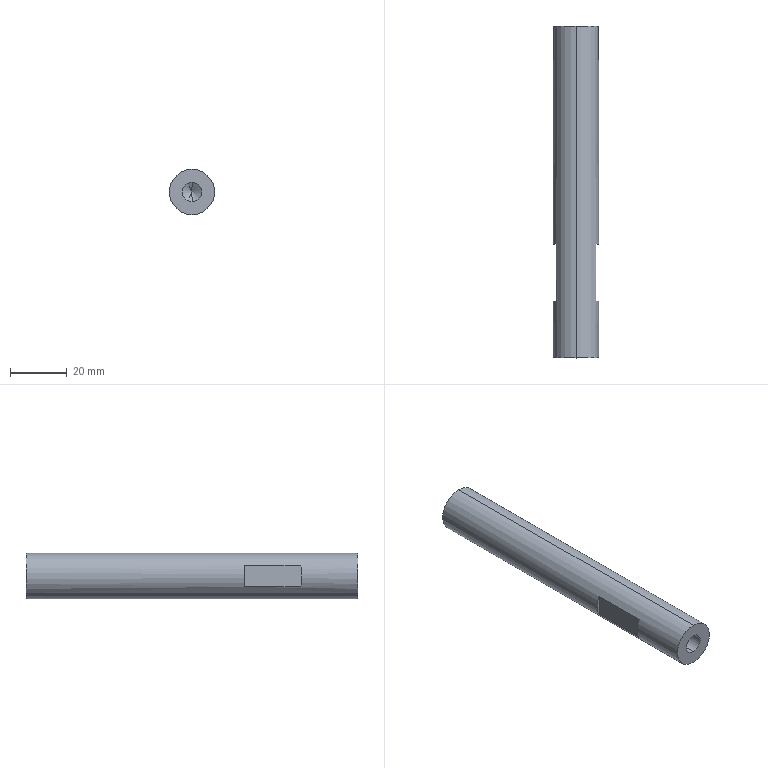Part | STEP file | 1 solid | 18 faces | box 16 x 117 x 16 mm | volume 21831 mm3 | plane 8 | cylinder 6 | cone 4 | commonest cylinder face diameters 6.8 x4 16 x2
STEP:
#1=CARTESIAN_POINT('',(0.,0.,0.));
#2=DIRECTION('',(0.,0.,1.));
#3=DIRECTION('',(1.,0.,0.));
#4=AXIS2_PLACEMENT_3D('',#1,#2,#3);
#5=CARTESIAN_POINT('',(0.,97.25,3.4));
#6=VERTEX_POINT('',#5);
#7=CARTESIAN_POINT('',(0.,117.,3.4));
#8=VERTEX_POINT('',#7);
#9=CARTESIAN_POINT('',(0.,117.,3.4));
#10=DIRECTION('',(0.,1.,0.));
#11=VECTOR('',#10,1.);
#12=LINE('',#9,#11);
#13=CARTESIAN_POINT('',(0.,117.,0.));
#14=DIRECTION('',(0.,1.,0.));
#15=DIRECTION('',(0.,0.,1.));
#16=AXIS2_PLACEMENT_3D('',#13,#14,#15);
#17=CYLINDRICAL_SURFACE('',#16,3.4);
#18=CARTESIAN_POINT('',(6.283,0.));
#19=DIRECTION('',(0.,1.));
#20=VECTOR('',#19,1.);
#21=LINE('',#18,#20);
#22=(GEOMETRIC_REPRESENTATION_CONTEXT(2)PARAMETRIC_REPRESENTATION_CONTEXT()REPRESENTATION_CONTEXT('',''));
#23=DEFINITIONAL_REPRESENTATION('',(#21),#22);
#24=PCURVE('',#17,#23);
#25=CARTESIAN_POINT('',(0.,117.,0.));
#26=DIRECTION('',(0.,1.,0.));
#27=DIRECTION('',(0.,0.,1.));
#28=AXIS2_PLACEMENT_3D('',#25,#26,#27);
#29=CYLINDRICAL_SURFACE('',#28,3.4);
#30=CARTESIAN_POINT('',(0.,0.));
#31=DIRECTION('',(0.,1.));
#32=VECTOR('',#31,1.);
#33=LINE('',#30,#32);
#34=(GEOMETRIC_REPRESENTATION_CONTEXT(2)PARAMETRIC_REPRESENTATION_CONTEXT()REPRESENTATION_CONTEXT('',''));
#35=DEFINITIONAL_REPRESENTATION('',(#33),#34);
#36=PCURVE('',#29,#35);
#37=SURFACE_CURVE('',#12,(#24,#36),.PCURVE_S1.);
#38=EDGE_CURVE('',#6,#8,#37,.T.);
#39=ORIENTED_EDGE('',*,*,#38,.T.);
#40=CARTESIAN_POINT('',(0.,117.,-3.4));
#41=VERTEX_POINT('',#40);
#42=CARTESIAN_POINT('',(0.,117.,0.));
#43=DIRECTION('',(0.,1.,0.));
#44=DIRECTION('',(0.,0.,1.));
#45=AXIS2_PLACEMENT_3D('',#42,#43,#44);
#46=CIRCLE('',#45,3.4);
#47=CARTESIAN_POINT('',(0.,0.));
#48=DIRECTION('',(1.,0.));
#49=VECTOR('',#48,1.);
#50=LINE('',#47,#49);
#51=(GEOMETRIC_REPRESENTATION_CONTEXT(2)PARAMETRIC_REPRESENTATION_CONTEXT()REPRESENTATION_CONTEXT('',''));
#52=DEFINITIONAL_REPRESENTATION('',(#50),#51);
#53=PCURVE('',#17,#52);
#54=CARTESIAN_POINT('',(8.,117.,0.));
#55=DIRECTION('',(0.,1.,0.));
#56=DIRECTION('',(0.,0.,1.));
#57=AXIS2_PLACEMENT_3D('',#54,#55,#56);
#58=PLANE('',#57);
#59=CARTESIAN_POINT('',(0.,-8.));
#60=DIRECTION('',(1.,0.));
#61=AXIS2_PLACEMENT_2D('',#59,#60);
#62=CIRCLE('',#61,3.4);
#63=(GEOMETRIC_REPRESENTATION_CONTEXT(2)PARAMETRIC_REPRESENTATION_CONTEXT()REPRESENTATION_CONTEXT('',''));
#64=DEFINITIONAL_REPRESENTATION('',(#62),#63);
#65=PCURVE('',#58,#64);
#66=SURFACE_CURVE('',#46,(#53,#65),.PCURVE_S1.);
#67=EDGE_CURVE('',#41,#8,#66,.T.);
#68=ORIENTED_EDGE('',*,*,#67,.F.);
#69=CARTESIAN_POINT('',(0.,97.25,-3.4));
#70=VERTEX_POINT('',#69);
#71=CARTESIAN_POINT('',(0.,117.,-3.4));
#72=DIRECTION('',(0.,1.,0.));
#73=VECTOR('',#72,1.);
#74=LINE('',#71,#73);
#75=CARTESIAN_POINT('',(3.142,0.));
#76=DIRECTION('',(0.,1.));
#77=VECTOR('',#76,1.);
#78=LINE('',#75,#77);
#79=(GEOMETRIC_REPRESENTATION_CONTEXT(2)PARAMETRIC_REPRESENTATION_CONTEXT()REPRESENTATION_CONTEXT('',''));
#80=DEFINITIONAL_REPRESENTATION('',(#78),#79);
#81=PCURVE('',#17,#80);
#82=CARTESIAN_POINT('',(3.142,0.));
#83=DIRECTION('',(0.,1.));
#84=VECTOR('',#83,1.);
#85=LINE('',#82,#84);
#86=(GEOMETRIC_REPRESENTATION_CONTEXT(2)PARAMETRIC_REPRESENTATION_CONTEXT()REPRESENTATION_CONTEXT('',''));
#87=DEFINITIONAL_REPRESENTATION('',(#85),#86);
#88=PCURVE('',#29,#87);
#89=SURFACE_CURVE('',#74,(#81,#88),.PCURVE_S1.);
#90=EDGE_CURVE('',#70,#41,#89,.T.);
#91=ORIENTED_EDGE('',*,*,#90,.F.);
#92=CARTESIAN_POINT('',(0.,97.25,0.));
#93=DIRECTION('',(0.,1.,0.));
#94=DIRECTION('',(0.,0.,1.));
#95=AXIS2_PLACEMENT_3D('',#92,#93,#94);
#96=CIRCLE('',#95,3.4);
#97=CARTESIAN_POINT('',(0.,-19.75));
#98=DIRECTION('',(1.,0.));
#99=VECTOR('',#98,1.);
#100=LINE('',#97,#99);
#101=(GEOMETRIC_REPRESENTATION_CONTEXT(2)PARAMETRIC_REPRESENTATION_CONTEXT()REPRESENTATION_CONTEXT('',''));
#102=DEFINITIONAL_REPRESENTATION('',(#100),#101);
#103=PCURVE('',#17,#102);
#104=CARTESIAN_POINT('',(0.,97.25,0.));
#105=DIRECTION('',(0.,1.,0.));
#106=DIRECTION('',(0.,0.,1.));
#107=AXIS2_PLACEMENT_3D('',#104,#105,#106);
#108=CONICAL_SURFACE('',#107,3.4,1.03);
#109=CARTESIAN_POINT('',(0.,0.));
#110=DIRECTION('',(1.,0.));
#111=VECTOR('',#110,1.);
#112=LINE('',#109,#111);
#113=(GEOMETRIC_REPRESENTATION_CONTEXT(2)PARAMETRIC_REPRESENTATION_CONTEXT()REPRESENTATION_CONTEXT('',''));
#114=DEFINITIONAL_REPRESENTATION('',(#112),#113);
#115=PCURVE('',#108,#114);
#116=SURFACE_CURVE('',#96,(#103,#115),.PCURVE_S1.);
#117=EDGE_CURVE('',#70,#6,#116,.T.);
#118=ORIENTED_EDGE('',*,*,#117,.T.);
#119=EDGE_LOOP('',(#39,#68,#91,#118));
#120=FACE_BOUND('',#119,.F.);
#121=ADVANCED_FACE('',(#120),#17,.F.);
#122=ORIENTED_EDGE('',*,*,#117,.F.);
#123=CARTESIAN_POINT('',(0.,95.207,0.));
#124=VERTEX_POINT('',#123);
#125=CARTESIAN_POINT('',(0.,97.25,-3.4));
#126=DIRECTION('',(0.,0.515,-0.8572));
#127=VECTOR('',#126,1.);
#128=LINE('',#125,#127);
#129=CARTESIAN_POINT('',(3.142,-2.043));
#130=CARTESIAN_POINT('',(3.142,-2.012));
#131=CARTESIAN_POINT('',(3.142,-1.95));
#132=CARTESIAN_POINT('',(3.142,-1.857));
#133=CARTESIAN_POINT('',(3.142,-1.764));
#134=CARTESIAN_POINT('',(3.142,-1.671));
#135=CARTESIAN_POINT('',(3.142,-1.579));
#136=CARTESIAN_POINT('',(3.142,-1.486));
#137=CARTESIAN_POINT('',(3.142,-1.393));
#138=CARTESIAN_POINT('',(3.142,-1.3));
#139=CARTESIAN_POINT('',(3.142,-1.207));
#140=CARTESIAN_POINT('',(3.142,-1.114));
#141=CARTESIAN_POINT('',(3.142,-1.021));
#142=CARTESIAN_POINT('',(3.142,-0.9286));
#143=CARTESIAN_POINT('',(3.142,-0.8357));
#144=CARTESIAN_POINT('',(3.142,-0.7429));
#145=CARTESIAN_POINT('',(3.142,-0.65));
#146=CARTESIAN_POINT('',(3.142,-0.5572));
#147=CARTESIAN_POINT('',(3.142,-0.4643));
#148=CARTESIAN_POINT('',(3.142,-0.3714));
#149=CARTESIAN_POINT('',(3.142,-0.2786));
#150=CARTESIAN_POINT('',(3.142,-0.1857));
#151=CARTESIAN_POINT('',(3.142,-0.09286));
#152=CARTESIAN_POINT('',(3.142,-0.03095));
#153=CARTESIAN_POINT('',(3.142,0.));
#154=B_SPLINE_CURVE_WITH_KNOTS('',3,(#129,#130,#131,#132,#133,#134,#135,#136,#137,#138,#139,#140,#141,#142,#143,#144,#145,#146,#147,#148,#149,#150,#151,#152,#153),.UNSPECIFIED.,.F.,.F.,(4,1,1,1,1,1,1,1,1,1,1,1,1,1,1,1,1,1,1,1,1,1,4),(-3.967,-3.786,-3.606,-3.426,-3.245,-3.065,-2.885,-2.704,-2.524,-2.344,-2.164,-1.983,-1.803,-1.623,-1.442,-1.262,-1.082,-0.9015,-0.7212,-0.5409,-0.3606,-0.1803,0.),.UNSPECIFIED.);
#155=(GEOMETRIC_REPRESENTATION_CONTEXT(2)PARAMETRIC_REPRESENTATION_CONTEXT()REPRESENTATION_CONTEXT('',''));
#156=DEFINITIONAL_REPRESENTATION('',(#154),#155);
#157=PCURVE('',#108,#156);
#158=CARTESIAN_POINT('',(0.,97.25,0.));
#159=DIRECTION('',(0.,1.,0.));
#160=DIRECTION('',(0.,0.,1.));
#161=AXIS2_PLACEMENT_3D('',#158,#159,#160);
#162=CONICAL_SURFACE('',#161,3.4,1.03);
#163=CARTESIAN_POINT('',(3.142,-2.043));
#164=CARTESIAN_POINT('',(3.142,-2.012));
#165=CARTESIAN_POINT('',(3.142,-1.95));
#166=CARTESIAN_POINT('',(3.142,-1.857));
#167=CARTESIAN_POINT('',(3.142,-1.764));
#168=CARTESIAN_POINT('',(3.142,-1.671));
#169=CARTESIAN_POINT('',(3.142,-1.579));
#170=CARTESIAN_POINT('',(3.142,-1.486));
#171=CARTESIAN_POINT('',(3.142,-1.393));
#172=CARTESIAN_POINT('',(3.142,-1.3));
#173=CARTESIAN_POINT('',(3.142,-1.207));
#174=CARTESIAN_POINT('',(3.142,-1.114));
#175=CARTESIAN_POINT('',(3.142,-1.021));
#176=CARTESIAN_POINT('',(3.142,-0.9286));
#177=CARTESIAN_POINT('',(3.142,-0.8357));
#178=CARTESIAN_POINT('',(3.142,-0.7429));
#179=CARTESIAN_POINT('',(3.142,-0.65));
#180=CARTESIAN_POINT('',(3.142,-0.5572));
#181=CARTESIAN_POINT('',(3.142,-0.4643));
#182=CARTESIAN_POINT('',(3.142,-0.3714));
#183=CARTESIAN_POINT('',(3.142,-0.2786));
#184=CARTESIAN_POINT('',(3.142,-0.1857));
#185=CARTESIAN_POINT('',(3.142,-0.09286));
#186=CARTESIAN_POINT('',(3.142,-0.03095));
#187=CARTESIAN_POINT('',(3.142,0.));
#188=B_SPLINE_CURVE_WITH_KNOTS('',3,(#163,#164,#165,#166,#167,#168,#169,#170,#171,#172,#173,#174,#175,#176,#177,#178,#179,#180,#181,#182,#183,#184,#185,#186,#187),.UNSPECIFIED.,.F.,.F.,(4,1,1,1,1,1,1,1,1,1,1,1,1,1,1,1,1,1,1,1,1,1,4),(-3.967,-3.786,-3.606,-3.426,-3.245,-3.065,-2.885,-2.704,-2.524,-2.344,-2.164,-1.983,-1.803,-1.623,-1.442,-1.262,-1.082,-0.9015,-0.7212,-0.5409,-0.3606,-0.1803,0.),.UNSPECIFIED.);
#189=(GEOMETRIC_REPRESENTATION_CONTEXT(2)PARAMETRIC_REPRESENTATION_CONTEXT()REPRESENTATION_CONTEXT('',''));
#190=DEFINITIONAL_REPRESENTATION('',(#188),#189);
#191=PCURVE('',#162,#190);
#192=SURFACE_CURVE('',#128,(#157,#191),.PCURVE_S1.);
#193=EDGE_CURVE('',#124,#70,#192,.T.);
#194=ORIENTED_EDGE('',*,*,#193,.F.);
#195=CARTESIAN_POINT('',(0.,97.25,3.4));
#196=DIRECTION('',(0.,0.515,0.8572));
#197=VECTOR('',#196,1.);
#198=LINE('',#195,#197);
#199=CARTESIAN_POINT('',(6.283,-2.043));
#200=CARTESIAN_POINT('',(6.283,-2.012));
#201=CARTESIAN_POINT('',(6.283,-1.95));
#202=CARTESIAN_POINT('',(6.283,-1.857));
#203=CARTESIAN_POINT('',(6.283,-1.764));
#204=CARTESIAN_POINT('',(6.283,-1.671));
#205=CARTESIAN_POINT('',(6.283,-1.579));
#206=CARTESIAN_POINT('',(6.283,-1.486));
#207=CARTESIAN_POINT('',(6.283,-1.393));
#208=CARTESIAN_POINT('',(6.283,-1.3));
#209=CARTESIAN_POINT('',(6.283,-1.207));
#210=CARTESIAN_POINT('',(6.283,-1.114));
#211=CARTESIAN_POINT('',(6.283,-1.021));
#212=CARTESIAN_POINT('',(6.283,-0.9286));
#213=CARTESIAN_POINT('',(6.283,-0.8357));
#214=CARTESIAN_POINT('',(6.283,-0.7429));
#215=CARTESIAN_POINT('',(6.283,-0.65));
#216=CARTESIAN_POINT('',(6.283,-0.5572));
#217=CARTESIAN_POINT('',(6.283,-0.4643));
#218=CARTESIAN_POINT('',(6.283,-0.3714));
#219=CARTESIAN_POINT('',(6.283,-0.2786));
#220=CARTESIAN_POINT('',(6.283,-0.1857));
#221=CARTESIAN_POINT('',(6.283,-0.09286));
#222=CARTESIAN_POINT('',(6.283,-0.03095));
#223=CARTESIAN_POINT('',(6.283,0.));
#224=B_SPLINE_CURVE_WITH_KNOTS('',3,(#199,#200,#201,#202,#203,#204,#205,#206,#207,#208,#209,#210,#211,#212,#213,#214,#215,#216,#217,#218,#219,#220,#221,#222,#223),.UNSPECIFIED.,.F.,.F.,(4,1,1,1,1,1,1,1,1,1,1,1,1,1,1,1,1,1,1,1,1,1,4),(-3.967,-3.786,-3.606,-3.426,-3.245,-3.065,-2.885,-2.704,-2.524,-2.344,-2.164,-1.983,-1.803,-1.623,-1.442,-1.262,-1.082,-0.9015,-0.7212,-0.5409,-0.3606,-0.1803,0.),.UNSPECIFIED.);
#225=(GEOMETRIC_REPRESENTATION_CONTEXT(2)PARAMETRIC_REPRESENTATION_CONTEXT()REPRESENTATION_CONTEXT('',''));
#226=DEFINITIONAL_REPRESENTATION('',(#224),#225);
#227=PCURVE('',#108,#226);
#228=CARTESIAN_POINT('',(0.,-2.043));
#229=CARTESIAN_POINT('',(0.,-2.012));
#230=CARTESIAN_POINT('',(0.,-1.95));
#231=CARTESIAN_POINT('',(0.,-1.857));
#232=CARTESIAN_POINT('',(0.,-1.764));
#233=CARTESIAN_POINT('',(0.,-1.671));
#234=CARTESIAN_POINT('',(0.,-1.579));
#235=CARTESIAN_POINT('',(0.,-1.486));
#236=CARTESIAN_POINT('',(0.,-1.393));
#237=CARTESIAN_POINT('',(0.,-1.3));
#238=CARTESIAN_POINT('',(0.,-1.207));
#239=CARTESIAN_POINT('',(0.,-1.114));
#240=CARTESIAN_POINT('',(0.,-1.021));
#241=CARTESIAN_POINT('',(0.,-0.9286));
#242=CARTESIAN_POINT('',(0.,-0.8357));
#243=CARTESIAN_POINT('',(0.,-0.7429));
#244=CARTESIAN_POINT('',(0.,-0.65));
#245=CARTESIAN_POINT('',(0.,-0.5572));
#246=CARTESIAN_POINT('',(0.,-0.4643));
#247=CARTESIAN_POINT('',(0.,-0.3714));
#248=CARTESIAN_POINT('',(0.,-0.2786));
#249=CARTESIAN_POINT('',(0.,-0.1857));
#250=CARTESIAN_POINT('',(0.,-0.09286));
#251=CARTESIAN_POINT('',(0.,-0.03095));
#252=CARTESIAN_POINT('',(0.,0.));
#253=B_SPLINE_CURVE_WITH_KNOTS('',3,(#228,#229,#230,#231,#232,#233,#234,#235,#236,#237,#238,#239,#240,#241,#242,#243,#244,#245,#246,#247,#248,#249,#250,#251,#252),.UNSPECIFIED.,.F.,.F.,(4,1,1,1,1,1,1,1,1,1,1,1,1,1,1,1,1,1,1,1,1,1,4),(-3.967,-3.786,-3.606,-3.426,-3.245,-3.065,-2.885,-2.704,-2.524,-2.344,-2.164,-1.983,-1.803,-1.623,-1.442,-1.262,-1.082,-0.9015,-0.7212,-0.5409,-0.3606,-0.1803,0.),.UNSPECIFIED.);
#254=(GEOMETRIC_REPRESENTATION_CONTEXT(2)PARAMETRIC_REPRESENTATION_CONTEXT()REPRESENTATION_CONTEXT('',''));
#255=DEFINITIONAL_REPRESENTATION('',(#253),#254);
#256=PCURVE('',#162,#255);
#257=SURFACE_CURVE('',#198,(#227,#256),.PCURVE_S1.);
#258=EDGE_CURVE('',#124,#6,#257,.T.);
#259=ORIENTED_EDGE('',*,*,#258,.T.);
#260=EDGE_LOOP('',(#122,#194,#259));
#261=FACE_BOUND('',#260,.F.);
#262=ADVANCED_FACE('',(#261),#108,.F.);
#263=CARTESIAN_POINT('',(0.,19.75,-3.4));
#264=VERTEX_POINT('',#263);
#265=CARTESIAN_POINT('',(0.,0.,-3.4));
#266=VERTEX_POINT('',#265);
#267=CARTESIAN_POINT('',(0.,0.,-3.4));
#268=DIRECTION('',(0.,-1.,0.));
#269=VECTOR('',#268,1.);
#270=LINE('',#267,#269);
#271=CARTESIAN_POINT('',(0.,0.,0.));
#272=DIRECTION('',(0.,-1.,0.));
#273=DIRECTION('',(0.,0.,-1.));
#274=AXIS2_PLACEMENT_3D('',#271,#272,#273);
#275=CYLINDRICAL_SURFACE('',#274,3.4);
#276=CARTESIAN_POINT('',(6.283,0.));
#277=DIRECTION('',(0.,1.));
#278=VECTOR('',#277,1.);
#279=LINE('',#276,#278);
#280=(GEOMETRIC_REPRESENTATION_CONTEXT(2)PARAMETRIC_REPRESENTATION_CONTEXT()REPRESENTATION_CONTEXT('',''));
#281=DEFINITIONAL_REPRESENTATION('',(#279),#280);
#282=PCURVE('',#275,#281);
#283=CARTESIAN_POINT('',(0.,0.,0.));
#284=DIRECTION('',(0.,-1.,0.));
#285=DIRECTION('',(0.,0.,-1.));
#286=AXIS2_PLACEMENT_3D('',#283,#284,#285);
#287=CYLINDRICAL_SURFACE('',#286,3.4);
#288=CARTESIAN_POINT('',(0.,0.));
#289=DIRECTION('',(0.,1.));
#290=VECTOR('',#289,1.);
#291=LINE('',#288,#290);
#292=(GEOMETRIC_REPRESENTATION_CONTEXT(2)PARAMETRIC_REPRESENTATION_CONTEXT()REPRESENTATION_CONTEXT('',''));
#293=DEFINITIONAL_REPRESENTATION('',(#291),#292);
#294=PCURVE('',#287,#293);
#295=SURFACE_CURVE('',#270,(#282,#294),.PCURVE_S1.);
#296=EDGE_CURVE('',#264,#266,#295,.T.);
#297=ORIENTED_EDGE('',*,*,#296,.T.);
#298=CARTESIAN_POINT('',(0.,0.,3.4));
#299=VERTEX_POINT('',#298);
#300=CARTESIAN_POINT('',(0.,0.,0.));
#301=DIRECTION('',(0.,-1.,0.));
#302=DIRECTION('',(0.,0.,-1.));
#303=AXIS2_PLACEMENT_3D('',#300,#301,#302);
#304=CIRCLE('',#303,3.4);
#305=CARTESIAN_POINT('',(0.,0.));
#306=DIRECTION('',(1.,0.));
#307=VECTOR('',#306,1.);
#308=LINE('',#305,#307);
#309=(GEOMETRIC_REPRESENTATION_CONTEXT(2)PARAMETRIC_REPRESENTATION_CONTEXT()REPRESENTATION_CONTEXT('',''));
#310=DEFINITIONAL_REPRESENTATION('',(#308),#309);
#311=PCURVE('',#275,#310);
#312=CARTESIAN_POINT('',(0.,0.,0.));
#313=DIRECTION('',(0.,-1.,0.));
#314=DIRECTION('',(0.,0.,-1.));
#315=AXIS2_PLACEMENT_3D('',#312,#313,#314);
#316=PLANE('',#315);
#317=CARTESIAN_POINT('',(0.,0.));
#318=DIRECTION('',(1.,0.));
#319=AXIS2_PLACEMENT_2D('',#317,#318);
#320=CIRCLE('',#319,3.4);
#321=(GEOMETRIC_REPRESENTATION_CONTEXT(2)PARAMETRIC_REPRESENTATION_CONTEXT()REPRESENTATION_CONTEXT('',''));
#322=DEFINITIONAL_REPRESENTATION('',(#320),#321);
#323=PCURVE('',#316,#322);
#324=SURFACE_CURVE('',#304,(#311,#323),.PCURVE_S1.);
#325=EDGE_CURVE('',#299,#266,#324,.T.);
#326=ORIENTED_EDGE('',*,*,#325,.F.);
#327=CARTESIAN_POINT('',(0.,19.75,3.4));
#328=VERTEX_POINT('',#327);
#329=CARTESIAN_POINT('',(0.,0.,3.4));
#330=DIRECTION('',(0.,-1.,0.));
#331=VECTOR('',#330,1.);
#332=LINE('',#329,#331);
#333=CARTESIAN_POINT('',(3.142,0.));
#334=DIRECTION('',(0.,1.));
#335=VECTOR('',#334,1.);
#336=LINE('',#333,#335);
#337=(GEOMETRIC_REPRESENTATION_CONTEXT(2)PARAMETRIC_REPRESENTATION_CONTEXT()REPRESENTATION_CONTEXT('',''));
#338=DEFINITIONAL_REPRESENTATION('',(#336),#337);
#339=PCURVE('',#275,#338);
#340=CARTESIAN_POINT('',(3.142,0.));
#341=DIRECTION('',(0.,1.));
#342=VECTOR('',#341,1.);
#343=LINE('',#340,#342);
#344=(GEOMETRIC_REPRESENTATION_CONTEXT(2)PARAMETRIC_REPRESENTATION_CONTEXT()REPRESENTATION_CONTEXT('',''));
#345=DEFINITIONAL_REPRESENTATION('',(#343),#344);
#346=PCURVE('',#287,#345);
#347=SURFACE_CURVE('',#332,(#339,#346),.PCURVE_S1.);
#348=EDGE_CURVE('',#328,#299,#347,.T.);
#349=ORIENTED_EDGE('',*,*,#348,.F.);
#350=CARTESIAN_POINT('',(0.,19.75,0.));
#351=DIRECTION('',(0.,-1.,0.));
#352=DIRECTION('',(0.,0.,-1.));
#353=AXIS2_PLACEMENT_3D('',#350,#351,#352);
#354=CIRCLE('',#353,3.4);
#355=CARTESIAN_POINT('',(0.,-19.75));
#356=DIRECTION('',(1.,0.));
#357=VECTOR('',#356,1.);
#358=LINE('',#355,#357);
#359=(GEOMETRIC_REPRESENTATION_CONTEXT(2)PARAMETRIC_REPRESENTATION_CONTEXT()REPRESENTATION_CONTEXT('',''));
#360=DEFINITIONAL_REPRESENTATION('',(#358),#359);
#361=PCURVE('',#275,#360);
#362=CARTESIAN_POINT('',(0.,19.75,0.));
#363=DIRECTION('',(0.,-1.,0.));
#364=DIRECTION('',(0.,0.,-1.));
#365=AXIS2_PLACEMENT_3D('',#362,#363,#364);
#366=CONICAL_SURFACE('',#365,3.4,1.03);
#367=CARTESIAN_POINT('',(0.,0.));
#368=DIRECTION('',(1.,0.));
#369=VECTOR('',#368,1.);
#370=LINE('',#367,#369);
#371=(GEOMETRIC_REPRESENTATION_CONTEXT(2)PARAMETRIC_REPRESENTATION_CONTEXT()REPRESENTATION_CONTEXT('',''));
#372=DEFINITIONAL_REPRESENTATION('',(#370),#371);
#373=PCURVE('',#366,#372);
#374=SURFACE_CURVE('',#354,(#361,#373),.PCURVE_S1.);
#375=EDGE_CURVE('',#328,#264,#374,.T.);
#376=ORIENTED_EDGE('',*,*,#375,.T.);
#377=EDGE_LOOP('',(#297,#326,#349,#376));
#378=FACE_BOUND('',#377,.F.);
#379=ADVANCED_FACE('',(#378),#275,.F.);
#380=ORIENTED_EDGE('',*,*,#375,.F.);
#381=CARTESIAN_POINT('',(0.,21.793,0.));
#382=VERTEX_POINT('',#381);
#383=CARTESIAN_POINT('',(0.,19.75,3.4));
#384=DIRECTION('',(0.,-0.515,0.8572));
#385=VECTOR('',#384,1.);
#386=LINE('',#383,#385);
#387=CARTESIAN_POINT('',(3.142,-2.043));
#388=CARTESIAN_POINT('',(3.142,-2.012));
#389=CARTESIAN_POINT('',(3.142,-1.95));
#390=CARTESIAN_POINT('',(3.142,-1.857));
#391=CARTESIAN_POINT('',(3.142,-1.764));
#392=CARTESIAN_POINT('',(3.142,-1.671));
#393=CARTESIAN_POINT('',(3.142,-1.579));
#394=CARTESIAN_POINT('',(3.142,-1.486));
#395=CARTESIAN_POINT('',(3.142,-1.393));
#396=CARTESIAN_POINT('',(3.142,-1.3));
#397=CARTESIAN_POINT('',(3.142,-1.207));
#398=CARTESIAN_POINT('',(3.142,-1.114));
#399=CARTESIAN_POINT('',(3.142,-1.021));
#400=CARTESIAN_POINT('',(3.142,-0.9286));
#401=CARTESIAN_POINT('',(3.142,-0.8357));
#402=CARTESIAN_POINT('',(3.142,-0.7429));
#403=CARTESIAN_POINT('',(3.142,-0.65));
#404=CARTESIAN_POINT('',(3.142,-0.5572));
#405=CARTESIAN_POINT('',(3.142,-0.4643));
#406=CARTESIAN_POINT('',(3.142,-0.3714));
#407=CARTESIAN_POINT('',(3.142,-0.2786));
#408=CARTESIAN_POINT('',(3.142,-0.1857));
#409=CARTESIAN_POINT('',(3.142,-0.09286));
#410=CARTESIAN_POINT('',(3.142,-0.03095));
#411=CARTESIAN_POINT('',(3.142,0.));
#412=B_SPLINE_CURVE_WITH_KNOTS('',3,(#387,#388,#389,#390,#391,#392,#393,#394,#395,#396,#397,#398,#399,#400,#401,#402,#403,#404,#405,#406,#407,#408,#409,#410,#411),.UNSPECIFIED.,.F.,.F.,(4,1,1,1,1,1,1,1,1,1,1,1,1,1,1,1,1,1,1,1,1,1,4),(-3.967,-3.786,-3.606,-3.426,-3.245,-3.065,-2.885,-2.704,-2.524,-2.344,-2.164,-1.983,-1.803,-1.623,-1.442,-1.262,-1.082,-0.9015,-0.7212,-0.5409,-0.3606,-0.1803,0.),.QUASI_UNIFORM_KNOTS.);
#413=(GEOMETRIC_REPRESENTATION_CONTEXT(2)PARAMETRIC_REPRESENTATION_CONTEXT()REPRESENTATION_CONTEXT('',''));
#414=DEFINITIONAL_REPRESENTATION('',(#412),#413);
#415=PCURVE('',#366,#414);
#416=CARTESIAN_POINT('',(0.,19.75,0.));
#417=DIRECTION('',(0.,-1.,0.));
#418=DIRECTION('',(0.,0.,-1.));
#419=AXIS2_PLACEMENT_3D('',#416,#417,#418);
#420=CONICAL_SURFACE('',#419,3.4,1.03);
#421=CARTESIAN_POINT('',(3.142,-2.043));
#422=CARTESIAN_POINT('',(3.142,-2.012));
#423=CARTESIAN_POINT('',(3.142,-1.95));
#424=CARTESIAN_POINT('',(3.142,-1.857));
#425=CARTESIAN_POINT('',(3.142,-1.764));
#426=CARTESIAN_POINT('',(3.142,-1.671));
#427=CARTESIAN_POINT('',(3.142,-1.579));
#428=CARTESIAN_POINT('',(3.142,-1.486));
#429=CARTESIAN_POINT('',(3.142,-1.393));
#430=CARTESIAN_POINT('',(3.142,-1.3));
#431=CARTESIAN_POINT('',(3.142,-1.207));
#432=CARTESIAN_POINT('',(3.142,-1.114));
#433=CARTESIAN_POINT('',(3.142,-1.021));
#434=CARTESIAN_POINT('',(3.142,-0.9286));
#435=CARTESIAN_POINT('',(3.142,-0.8357));
#436=CARTESIAN_POINT('',(3.142,-0.7429));
#437=CARTESIAN_POINT('',(3.142,-0.65));
#438=CARTESIAN_POINT('',(3.142,-0.5572));
#439=CARTESIAN_POINT('',(3.142,-0.4643));
#440=CARTESIAN_POINT('',(3.142,-0.3714));
#441=CARTESIAN_POINT('',(3.142,-0.2786));
#442=CARTESIAN_POINT('',(3.142,-0.1857));
#443=CARTESIAN_POINT('',(3.142,-0.09286));
#444=CARTESIAN_POINT('',(3.142,-0.03095));
#445=CARTESIAN_POINT('',(3.142,0.));
#446=B_SPLINE_CURVE_WITH_KNOTS('',3,(#421,#422,#423,#424,#425,#426,#427,#428,#429,#430,#431,#432,#433,#434,#435,#436,#437,#438,#439,#440,#441,#442,#443,#444,#445),.UNSPECIFIED.,.F.,.F.,(4,1,1,1,1,1,1,1,1,1,1,1,1,1,1,1,1,1,1,1,1,1,4),(-3.967,-3.786,-3.606,-3.426,-3.245,-3.065,-2.885,-2.704,-2.524,-2.344,-2.164,-1.983,-1.803,-1.623,-1.442,-1.262,-1.082,-0.9015,-0.7212,-0.5409,-0.3606,-0.1803,0.),.QUASI_UNIFORM_KNOTS.);
#447=(GEOMETRIC_REPRESENTATION_CONTEXT(2)PARAMETRIC_REPRESENTATION_CONTEXT()REPRESENTATION_CONTEXT('',''));
#448=DEFINITIONAL_REPRESENTATION('',(#446),#447);
#449=PCURVE('',#420,#448);
#450=SURFACE_CURVE('',#386,(#415,#449),.PCURVE_S1.);
#451=EDGE_CURVE('',#382,#328,#450,.T.);
#452=ORIENTED_EDGE('',*,*,#451,.F.);
#453=CARTESIAN_POINT('',(0.,19.75,-3.4));
#454=DIRECTION('',(0.,-0.515,-0.8572));
#455=VECTOR('',#454,1.);
#456=LINE('',#453,#455);
#457=CARTESIAN_POINT('',(6.283,-2.043));
#458=CARTESIAN_POINT('',(6.283,-2.012));
#459=CARTESIAN_POINT('',(6.283,-1.95));
#460=CARTESIAN_POINT('',(6.283,-1.857));
#461=CARTESIAN_POINT('',(6.283,-1.764));
#462=CARTESIAN_POINT('',(6.283,-1.671));
#463=CARTESIAN_POINT('',(6.283,-1.579));
#464=CARTESIAN_POINT('',(6.283,-1.486));
#465=CARTESIAN_POINT('',(6.283,-1.393));
#466=CARTESIAN_POINT('',(6.283,-1.3));
#467=CARTESIAN_POINT('',(6.283,-1.207));
#468=CARTESIAN_POINT('',(6.283,-1.114));
#469=CARTESIAN_POINT('',(6.283,-1.021));
#470=CARTESIAN_POINT('',(6.283,-0.9286));
#471=CARTESIAN_POINT('',(6.283,-0.8357));
#472=CARTESIAN_POINT('',(6.283,-0.7429));
#473=CARTESIAN_POINT('',(6.283,-0.65));
#474=CARTESIAN_POINT('',(6.283,-0.5572));
#475=CARTESIAN_POINT('',(6.283,-0.4643));
#476=CARTESIAN_POINT('',(6.283,-0.3714));
#477=CARTESIAN_POINT('',(6.283,-0.2786));
#478=CARTESIAN_POINT('',(6.283,-0.1857));
#479=CARTESIAN_POINT('',(6.283,-0.09286));
#480=CARTESIAN_POINT('',(6.283,-0.03095));
#481=CARTESIAN_POINT('',(6.283,0.));
#482=B_SPLINE_CURVE_WITH_KNOTS('',3,(#457,#458,#459,#460,#461,#462,#463,#464,#465,#466,#467,#468,#469,#470,#471,#472,#473,#474,#475,#476,#477,#478,#479,#480,#481),.UNSPECIFIED.,.F.,.F.,(4,1,1,1,1,1,1,1,1,1,1,1,1,1,1,1,1,1,1,1,1,1,4),(-3.967,-3.786,-3.606,-3.426,-3.245,-3.065,-2.885,-2.704,-2.524,-2.344,-2.164,-1.983,-1.803,-1.623,-1.442,-1.262,-1.082,-0.9015,-0.7212,-0.5409,-0.3606,-0.1803,0.),.QUASI_UNIFORM_KNOTS.);
#483=(GEOMETRIC_REPRESENTATION_CONTEXT(2)PARAMETRIC_REPRESENTATION_CONTEXT()REPRESENTATION_CONTEXT('',''));
#484=DEFINITIONAL_REPRESENTATION('',(#482),#483);
#485=PCURVE('',#366,#484);
#486=CARTESIAN_POINT('',(0.,-2.043));
#487=CARTESIAN_POINT('',(0.,-2.012));
#488=CARTESIAN_POINT('',(0.,-1.95));
#489=CARTESIAN_POINT('',(0.,-1.857));
#490=CARTESIAN_POINT('',(0.,-1.764));
#491=CARTESIAN_POINT('',(0.,-1.671));
#492=CARTESIAN_POINT('',(0.,-1.579));
#493=CARTESIAN_POINT('',(0.,-1.486));
#494=CARTESIAN_POINT('',(0.,-1.393));
#495=CARTESIAN_POINT('',(0.,-1.3));
#496=CARTESIAN_POINT('',(0.,-1.207));
#497=CARTESIAN_POINT('',(0.,-1.114));
#498=CARTESIAN_POINT('',(0.,-1.021));
#499=CARTESIAN_POINT('',(0.,-0.9286));
#500=CARTESIAN_POINT('',(0.,-0.8357));
#501=CARTESIAN_POINT('',(0.,-0.7429));
#502=CARTESIAN_POINT('',(0.,-0.65));
#503=CARTESIAN_POINT('',(0.,-0.5572));
#504=CARTESIAN_POINT('',(0.,-0.4643));
#505=CARTESIAN_POINT('',(0.,-0.3714));
#506=CARTESIAN_POINT('',(0.,-0.2786));
#507=CARTESIAN_POINT('',(0.,-0.1857));
#508=CARTESIAN_POINT('',(0.,-0.09286));
#509=CARTESIAN_POINT('',(0.,-0.03095));
#510=CARTESIAN_POINT('',(0.,0.));
#511=B_SPLINE_CURVE_WITH_KNOTS('',3,(#486,#487,#488,#489,#490,#491,#492,#493,#494,#495,#496,#497,#498,#499,#500,#501,#502,#503,#504,#505,#506,#507,#508,#509,#510),.UNSPECIFIED.,.F.,.F.,(4,1,1,1,1,1,1,1,1,1,1,1,1,1,1,1,1,1,1,1,1,1,4),(-3.967,-3.786,-3.606,-3.426,-3.245,-3.065,-2.885,-2.704,-2.524,-2.344,-2.164,-1.983,-1.803,-1.623,-1.442,-1.262,-1.082,-0.9015,-0.7212,-0.5409,-0.3606,-0.1803,0.),.QUASI_UNIFORM_KNOTS.);
#512=(GEOMETRIC_REPRESENTATION_CONTEXT(2)PARAMETRIC_REPRESENTATION_CONTEXT()REPRESENTATION_CONTEXT('',''));
#513=DEFINITIONAL_REPRESENTATION('',(#511),#512);
#514=PCURVE('',#420,#513);
#515=SURFACE_CURVE('',#456,(#485,#514),.PCURVE_S1.);
#516=EDGE_CURVE('',#382,#264,#515,.T.);
#517=ORIENTED_EDGE('',*,*,#516,.T.);
#518=EDGE_LOOP('',(#380,#452,#517));
#519=FACE_BOUND('',#518,.F.);
#520=ADVANCED_FACE('',(#519),#366,.F.);
#521=CARTESIAN_POINT('',(7.,20.,3.873));
#522=VERTEX_POINT('',#521);
#523=CARTESIAN_POINT('',(7.,20.,-3.873));
#524=VERTEX_POINT('',#523);
#525=CARTESIAN_POINT('',(0.,20.,0.));
#526=DIRECTION('',(0.,1.,0.));
#527=DIRECTION('',(1.,0.,0.));
#528=AXIS2_PLACEMENT_3D('',#525,#526,#527);
#529=CIRCLE('',#528,8.);
#530=CARTESIAN_POINT('',(0.,0.,0.));
#531=DIRECTION('',(0.,-1.,0.));
#532=DIRECTION('',(0.,0.,-1.));
#533=AXIS2_PLACEMENT_3D('',#530,#531,#532);
#534=CYLINDRICAL_SURFACE('',#533,8.);
#535=CARTESIAN_POINT('',(7.854,-20.));
#536=DIRECTION('',(-1.,0.));
#537=VECTOR('',#536,1.);
#538=LINE('',#535,#537);
#539=(GEOMETRIC_REPRESENTATION_CONTEXT(2)PARAMETRIC_REPRESENTATION_CONTEXT()REPRESENTATION_CONTEXT('',''));
#540=DEFINITIONAL_REPRESENTATION('',(#538),#539);
#541=PCURVE('',#534,#540);
#542=CARTESIAN_POINT('',(13.,20.,-10.));
#543=DIRECTION('',(0.,-1.,0.));
#544=DIRECTION('',(1.,0.,0.));
#545=AXIS2_PLACEMENT_3D('',#542,#543,#544);
#546=PLANE('',#545);
#547=CARTESIAN_POINT('',(-5.,10.));
#548=CARTESIAN_POINT('',(-5.,-3.856));
#549=CARTESIAN_POINT('',(-17.,3.072));
#550=CARTESIAN_POINT('',(-29.,10.));
#551=CARTESIAN_POINT('',(-17.,16.928));
#552=CARTESIAN_POINT('',(-5.,23.856));
#553=CARTESIAN_POINT('',(-5.,10.));
#554=(BOUNDED_CURVE()B_SPLINE_CURVE(2,(#547,#548,#549,#550,#551,#552,#553),.UNSPECIFIED.,.T.,.F.)B_SPLINE_CURVE_WITH_KNOTS((1,2,2,2,2,1),(-2.094,0.,2.094,4.189,6.283,8.378),.UNSPECIFIED.)CURVE()GEOMETRIC_REPRESENTATION_ITEM()RATIONAL_B_SPLINE_CURVE((1.,0.5,1.,0.5,1.,0.5,1.))REPRESENTATION_ITEM(''));
#555=(GEOMETRIC_REPRESENTATION_CONTEXT(2)PARAMETRIC_REPRESENTATION_CONTEXT()REPRESENTATION_CONTEXT('',''));
#556=DEFINITIONAL_REPRESENTATION('',(#554),#555);
#557=PCURVE('',#546,#556);
#558=SURFACE_CURVE('',#529,(#541,#557),.PCURVE_S1.);
#559=EDGE_CURVE('',#522,#524,#558,.T.);
#560=ORIENTED_EDGE('',*,*,#559,.F.);
#561=CARTESIAN_POINT('',(7.,40.,3.873));
#562=VERTEX_POINT('',#561);
#563=CARTESIAN_POINT('',(7.,0.,3.873));
#564=DIRECTION('',(0.,-1.,0.));
#565=VECTOR('',#564,1.);
#566=LINE('',#563,#565);
#567=CARTESIAN_POINT('',(2.076,0.));
#568=DIRECTION('',(0.,1.));
#569=VECTOR('',#568,1.);
#570=LINE('',#567,#569);
#571=(GEOMETRIC_REPRESENTATION_CONTEXT(2)PARAMETRIC_REPRESENTATION_CONTEXT()REPRESENTATION_CONTEXT('',''));
#572=DEFINITIONAL_REPRESENTATION('',(#570),#571);
#573=PCURVE('',#534,#572);
#574=CARTESIAN_POINT('',(7.,20.,-10.));
#575=DIRECTION('',(-1.,0.,0.));
#576=DIRECTION('',(0.,0.,1.));
#577=AXIS2_PLACEMENT_3D('',#574,#575,#576);
#578=PLANE('',#577);
#579=CARTESIAN_POINT('',(13.873,-20.));
#580=DIRECTION('',(0.,-1.));
#581=VECTOR('',#580,1.);
#582=LINE('',#579,#581);
#583=(GEOMETRIC_REPRESENTATION_CONTEXT(2)PARAMETRIC_REPRESENTATION_CONTEXT()REPRESENTATION_CONTEXT('',''));
#584=DEFINITIONAL_REPRESENTATION('',(#582),#583);
#585=PCURVE('',#578,#584);
#586=SURFACE_CURVE('',#566,(#573,#585),.PCURVE_S1.);
#587=EDGE_CURVE('',#562,#522,#586,.T.);
#588=ORIENTED_EDGE('',*,*,#587,.F.);
#589=CARTESIAN_POINT('',(7.,40.,-3.873));
#590=VERTEX_POINT('',#589);
#591=CARTESIAN_POINT('',(0.,40.,0.));
#592=DIRECTION('',(0.,-1.,0.));
#593=DIRECTION('',(0.,0.,1.));
#594=AXIS2_PLACEMENT_3D('',#591,#592,#593);
#595=CIRCLE('',#594,8.);
#596=CARTESIAN_POINT('',(-3.142,-40.));
#597=DIRECTION('',(1.,0.));
#598=VECTOR('',#597,1.);
#599=LINE('',#596,#598);
#600=(GEOMETRIC_REPRESENTATION_CONTEXT(2)PARAMETRIC_REPRESENTATION_CONTEXT()REPRESENTATION_CONTEXT('',''));
#601=DEFINITIONAL_REPRESENTATION('',(#599),#600);
#602=PCURVE('',#534,#601);
#603=CARTESIAN_POINT('',(13.,40.,-10.));
#604=DIRECTION('',(0.,1.,0.));
#605=DIRECTION('',(0.,0.,1.));
#606=AXIS2_PLACEMENT_3D('',#603,#604,#605);
#607=PLANE('',#606);
#608=CARTESIAN_POINT('',(18.,-13.));
#609=CARTESIAN_POINT('',(18.,-26.856));
#610=CARTESIAN_POINT('',(6.,-19.928));
#611=CARTESIAN_POINT('',(-6.,-13.));
#612=CARTESIAN_POINT('',(6.,-6.072));
#613=CARTESIAN_POINT('',(18.,0.8564));
#614=CARTESIAN_POINT('',(18.,-13.));
#615=(BOUNDED_CURVE()B_SPLINE_CURVE(2,(#608,#609,#610,#611,#612,#613,#614),.UNSPECIFIED.,.T.,.F.)B_SPLINE_CURVE_WITH_KNOTS((1,2,2,2,2,1),(-2.094,0.,2.094,4.189,6.283,8.378),.UNSPECIFIED.)CURVE()GEOMETRIC_REPRESENTATION_ITEM()RATIONAL_B_SPLINE_CURVE((1.,0.5,1.,0.5,1.,0.5,1.))REPRESENTATION_ITEM(''));
#616=(GEOMETRIC_REPRESENTATION_CONTEXT(2)PARAMETRIC_REPRESENTATION_CONTEXT()REPRESENTATION_CONTEXT('',''));
#617=DEFINITIONAL_REPRESENTATION('',(#615),#616);
#618=PCURVE('',#607,#617);
#619=SURFACE_CURVE('',#595,(#602,#618),.PCURVE_S1.);
#620=EDGE_CURVE('',#590,#562,#619,.T.);
#621=ORIENTED_EDGE('',*,*,#620,.F.);
#622=CARTESIAN_POINT('',(7.,0.,-3.873));
#623=DIRECTION('',(0.,1.,0.));
#624=VECTOR('',#623,1.);
#625=LINE('',#622,#624);
#626=CARTESIAN_POINT('',(1.065,0.));
#627=DIRECTION('',(0.,-1.));
#628=VECTOR('',#627,1.);
#629=LINE('',#626,#628);
#630=(GEOMETRIC_REPRESENTATION_CONTEXT(2)PARAMETRIC_REPRESENTATION_CONTEXT()REPRESENTATION_CONTEXT('',''));
#631=DEFINITIONAL_REPRESENTATION('',(#629),#630);
#632=PCURVE('',#534,#631);
#633=CARTESIAN_POINT('',(6.127,-20.));
#634=DIRECTION('',(0.,1.));
#635=VECTOR('',#634,1.);
#636=LINE('',#633,#635);
#637=(GEOMETRIC_REPRESENTATION_CONTEXT(2)PARAMETRIC_REPRESENTATION_CONTEXT()REPRESENTATION_CONTEXT('',''));
#638=DEFINITIONAL_REPRESENTATION('',(#636),#637);
#639=PCURVE('',#578,#638);
#640=SURFACE_CURVE('',#625,(#632,#639),.PCURVE_S1.);
#641=EDGE_CURVE('',#524,#590,#640,.T.);
#642=ORIENTED_EDGE('',*,*,#641,.F.);
#643=EDGE_LOOP('',(#560,#588,#621,#642));
#644=FACE_BOUND('',#643,.T.);
#645=CARTESIAN_POINT('',(0.,117.,-8.));
#646=VERTEX_POINT('',#645);
#647=CARTESIAN_POINT('',(0.,117.,8.));
#648=VERTEX_POINT('',#647);
#649=CARTESIAN_POINT('',(0.,117.,0.));
#650=DIRECTION('',(0.,-1.,0.));
#651=DIRECTION('',(0.,0.,-1.));
#652=AXIS2_PLACEMENT_3D('',#649,#650,#651);
#653=CIRCLE('',#652,8.);
#654=CARTESIAN_POINT('',(0.,-117.));
#655=DIRECTION('',(1.,0.));
#656=VECTOR('',#655,1.);
#657=LINE('',#654,#656);
#658=(GEOMETRIC_REPRESENTATION_CONTEXT(2)PARAMETRIC_REPRESENTATION_CONTEXT()REPRESENTATION_CONTEXT('',''));
#659=DEFINITIONAL_REPRESENTATION('',(#657),#658);
#660=PCURVE('',#534,#659);
#661=CARTESIAN_POINT('',(-8.,-8.));
#662=CARTESIAN_POINT('',(-8.,5.856));
#663=CARTESIAN_POINT('',(4.,-1.072));
#664=CARTESIAN_POINT('',(16.,-8.));
#665=CARTESIAN_POINT('',(4.,-14.928));
#666=CARTESIAN_POINT('',(-8.,-21.856));
#667=CARTESIAN_POINT('',(-8.,-8.));
#668=(BOUNDED_CURVE()B_SPLINE_CURVE(2,(#661,#662,#663,#664,#665,#666,#667),.UNSPECIFIED.,.T.,.F.)B_SPLINE_CURVE_WITH_KNOTS((1,2,2,2,2,1),(-2.094,0.,2.094,4.189,6.283,8.378),.UNSPECIFIED.)CURVE()GEOMETRIC_REPRESENTATION_ITEM()RATIONAL_B_SPLINE_CURVE((1.,0.5,1.,0.5,1.,0.5,1.))REPRESENTATION_ITEM(''));
#669=(GEOMETRIC_REPRESENTATION_CONTEXT(2)PARAMETRIC_REPRESENTATION_CONTEXT()REPRESENTATION_CONTEXT('',''));
#670=DEFINITIONAL_REPRESENTATION('',(#668),#669);
#671=PCURVE('',#58,#670);
#672=SURFACE_CURVE('',#653,(#660,#671),.PCURVE_S1.);
#673=EDGE_CURVE('',#646,#648,#672,.T.);
#674=ORIENTED_EDGE('',*,*,#673,.T.);
#675=CARTESIAN_POINT('',(0.,0.,8.));
#676=VERTEX_POINT('',#675);
#677=CARTESIAN_POINT('',(0.,0.,8.));
#678=DIRECTION('',(0.,-1.,0.));
#679=VECTOR('',#678,1.);
#680=LINE('',#677,#679);
#681=CARTESIAN_POINT('',(3.142,0.));
#682=DIRECTION('',(0.,1.));
#683=VECTOR('',#682,1.);
#684=LINE('',#681,#683);
#685=(GEOMETRIC_REPRESENTATION_CONTEXT(2)PARAMETRIC_REPRESENTATION_CONTEXT()REPRESENTATION_CONTEXT('',''));
#686=DEFINITIONAL_REPRESENTATION('',(#684),#685);
#687=PCURVE('',#534,#686);
#688=CARTESIAN_POINT('',(0.,0.,0.));
#689=DIRECTION('',(0.,-1.,0.));
#690=DIRECTION('',(0.,0.,-1.));
#691=AXIS2_PLACEMENT_3D('',#688,#689,#690);
#692=CYLINDRICAL_SURFACE('',#691,8.);
#693=CARTESIAN_POINT('',(3.142,0.));
#694=DIRECTION('',(0.,1.));
#695=VECTOR('',#694,1.);
#696=LINE('',#693,#695);
#697=(GEOMETRIC_REPRESENTATION_CONTEXT(2)PARAMETRIC_REPRESENTATION_CONTEXT()REPRESENTATION_CONTEXT('',''));
#698=DEFINITIONAL_REPRESENTATION('',(#696),#697);
#699=PCURVE('',#692,#698);
#700=SURFACE_CURVE('',#680,(#687,#699),.PCURVE_S1.);
#701=EDGE_CURVE('',#648,#676,#700,.T.);
#702=ORIENTED_EDGE('',*,*,#701,.T.);
#703=CARTESIAN_POINT('',(0.,0.,-8.));
#704=VERTEX_POINT('',#703);
#705=CARTESIAN_POINT('',(0.,0.,0.));
#706=DIRECTION('',(0.,-1.,0.));
#707=DIRECTION('',(0.,0.,-1.));
#708=AXIS2_PLACEMENT_3D('',#705,#706,#707);
#709=CIRCLE('',#708,8.);
#710=CARTESIAN_POINT('',(0.,0.));
#711=DIRECTION('',(1.,0.));
#712=VECTOR('',#711,1.);
#713=LINE('',#710,#712);
#714=(GEOMETRIC_REPRESENTATION_CONTEXT(2)PARAMETRIC_REPRESENTATION_CONTEXT()REPRESENTATION_CONTEXT('',''));
#715=DEFINITIONAL_REPRESENTATION('',(#713),#714);
#716=PCURVE('',#534,#715);
#717=CARTESIAN_POINT('',(0.,0.));
#718=DIRECTION('',(1.,0.));
#719=AXIS2_PLACEMENT_2D('',#717,#718);
#720=CIRCLE('',#719,8.);
#721=(GEOMETRIC_REPRESENTATION_CONTEXT(2)PARAMETRIC_REPRESENTATION_CONTEXT()REPRESENTATION_CONTEXT('',''));
#722=DEFINITIONAL_REPRESENTATION('',(#720),#721);
#723=PCURVE('',#316,#722);
#724=SURFACE_CURVE('',#709,(#716,#723),.PCURVE_S1.);
#725=EDGE_CURVE('',#704,#676,#724,.T.);
#726=ORIENTED_EDGE('',*,*,#725,.F.);
#727=CARTESIAN_POINT('',(0.,0.,-8.));
#728=DIRECTION('',(0.,-1.,0.));
#729=VECTOR('',#728,1.);
#730=LINE('',#727,#729);
#731=CARTESIAN_POINT('',(0.,0.));
#732=DIRECTION('',(0.,1.));
#733=VECTOR('',#732,1.);
#734=LINE('',#731,#733);
#735=(GEOMETRIC_REPRESENTATION_CONTEXT(2)PARAMETRIC_REPRESENTATION_CONTEXT()REPRESENTATION_CONTEXT('',''));
#736=DEFINITIONAL_REPRESENTATION('',(#734),#735);
#737=PCURVE('',#534,#736);
#738=CARTESIAN_POINT('',(6.283,0.));
#739=DIRECTION('',(0.,1.));
#740=VECTOR('',#739,1.);
#741=LINE('',#738,#740);
#742=(GEOMETRIC_REPRESENTATION_CONTEXT(2)PARAMETRIC_REPRESENTATION_CONTEXT()REPRESENTATION_CONTEXT('',''));
#743=DEFINITIONAL_REPRESENTATION('',(#741),#742);
#744=PCURVE('',#692,#743);
#745=SURFACE_CURVE('',#730,(#737,#744),.PCURVE_S1.);
#746=EDGE_CURVE('',#646,#704,#745,.T.);
#747=ORIENTED_EDGE('',*,*,#746,.F.);
#748=EDGE_LOOP('',(#674,#702,#726,#747));
#749=FACE_BOUND('',#748,.T.);
#750=ADVANCED_FACE('',(#644,#749),#534,.T.);
#751=CARTESIAN_POINT('',(0.,0.,0.));
#752=DIRECTION('',(0.,-1.,0.));
#753=DIRECTION('',(0.,0.,-1.));
#754=AXIS2_PLACEMENT_3D('',#751,#752,#753);
#755=CIRCLE('',#754,3.4);
#756=CARTESIAN_POINT('',(0.,0.));
#757=DIRECTION('',(1.,0.));
#758=AXIS2_PLACEMENT_2D('',#756,#757);
#759=CIRCLE('',#758,3.4);
#760=(GEOMETRIC_REPRESENTATION_CONTEXT(2)PARAMETRIC_REPRESENTATION_CONTEXT()REPRESENTATION_CONTEXT('',''));
#761=DEFINITIONAL_REPRESENTATION('',(#759),#760);
#762=PCURVE('',#316,#761);
#763=CARTESIAN_POINT('',(0.,0.));
#764=DIRECTION('',(1.,0.));
#765=VECTOR('',#764,1.);
#766=LINE('',#763,#765);
#767=(GEOMETRIC_REPRESENTATION_CONTEXT(2)PARAMETRIC_REPRESENTATION_CONTEXT()REPRESENTATION_CONTEXT('',''));
#768=DEFINITIONAL_REPRESENTATION('',(#766),#767);
#769=PCURVE('',#287,#768);
#770=SURFACE_CURVE('',#755,(#762,#769),.PCURVE_S1.);
#771=EDGE_CURVE('',#266,#299,#770,.T.);
#772=ORIENTED_EDGE('',*,*,#771,.F.);
#773=ORIENTED_EDGE('',*,*,#325,.F.);
#774=EDGE_LOOP('',(#772,#773));
#775=FACE_BOUND('',#774,.T.);
#776=ORIENTED_EDGE('',*,*,#725,.T.);
#777=CARTESIAN_POINT('',(0.,0.,0.));
#778=DIRECTION('',(0.,-1.,0.));
#779=DIRECTION('',(0.,0.,-1.));
#780=AXIS2_PLACEMENT_3D('',#777,#778,#779);
#781=CIRCLE('',#780,8.);
#782=CARTESIAN_POINT('',(0.,0.));
#783=DIRECTION('',(1.,0.));
#784=AXIS2_PLACEMENT_2D('',#782,#783);
#785=CIRCLE('',#784,8.);
#786=(GEOMETRIC_REPRESENTATION_CONTEXT(2)PARAMETRIC_REPRESENTATION_CONTEXT()REPRESENTATION_CONTEXT('',''));
#787=DEFINITIONAL_REPRESENTATION('',(#785),#786);
#788=PCURVE('',#316,#787);
#789=CARTESIAN_POINT('',(0.,0.));
#790=DIRECTION('',(1.,0.));
#791=VECTOR('',#790,1.);
#792=LINE('',#789,#791);
#793=(GEOMETRIC_REPRESENTATION_CONTEXT(2)PARAMETRIC_REPRESENTATION_CONTEXT()REPRESENTATION_CONTEXT('',''));
#794=DEFINITIONAL_REPRESENTATION('',(#792),#793);
#795=PCURVE('',#692,#794);
#796=SURFACE_CURVE('',#781,(#788,#795),.PCURVE_S1.);
#797=EDGE_CURVE('',#676,#704,#796,.T.);
#798=ORIENTED_EDGE('',*,*,#797,.T.);
#799=EDGE_LOOP('',(#776,#798));
#800=FACE_BOUND('',#799,.T.);
#801=ADVANCED_FACE('',(#775,#800),#316,.T.);
#802=ORIENTED_EDGE('',*,*,#701,.F.);
#803=CARTESIAN_POINT('',(0.,117.,0.));
#804=DIRECTION('',(0.,-1.,0.));
#805=DIRECTION('',(0.,0.,-1.));
#806=AXIS2_PLACEMENT_3D('',#803,#804,#805);
#807=CIRCLE('',#806,8.);
#808=CARTESIAN_POINT('',(0.,-117.));
#809=DIRECTION('',(1.,0.));
#810=VECTOR('',#809,1.);
#811=LINE('',#808,#810);
#812=(GEOMETRIC_REPRESENTATION_CONTEXT(2)PARAMETRIC_REPRESENTATION_CONTEXT()REPRESENTATION_CONTEXT('',''));
#813=DEFINITIONAL_REPRESENTATION('',(#811),#812);
#814=PCURVE('',#692,#813);
#815=CARTESIAN_POINT('',(-8.,-8.));
#816=CARTESIAN_POINT('',(-8.,5.856));
#817=CARTESIAN_POINT('',(4.,-1.072));
#818=CARTESIAN_POINT('',(16.,-8.));
#819=CARTESIAN_POINT('',(4.,-14.928));
#820=CARTESIAN_POINT('',(-8.,-21.856));
#821=CARTESIAN_POINT('',(-8.,-8.));
#822=(BOUNDED_CURVE()B_SPLINE_CURVE(2,(#815,#816,#817,#818,#819,#820,#821),.UNSPECIFIED.,.T.,.F.)B_SPLINE_CURVE_WITH_KNOTS((1,2,2,2,2,1),(-2.094,0.,2.094,4.189,6.283,8.378),.UNSPECIFIED.)CURVE()GEOMETRIC_REPRESENTATION_ITEM()RATIONAL_B_SPLINE_CURVE((1.,0.5,1.,0.5,1.,0.5,1.))REPRESENTATION_ITEM(''));
#823=(GEOMETRIC_REPRESENTATION_CONTEXT(2)PARAMETRIC_REPRESENTATION_CONTEXT()REPRESENTATION_CONTEXT('',''));
#824=DEFINITIONAL_REPRESENTATION('',(#822),#823);
#825=PCURVE('',#58,#824);
#826=SURFACE_CURVE('',#807,(#814,#825),.PCURVE_S1.);
#827=EDGE_CURVE('',#648,#646,#826,.T.);
#828=ORIENTED_EDGE('',*,*,#827,.T.);
#829=ORIENTED_EDGE('',*,*,#746,.T.);
#830=ORIENTED_EDGE('',*,*,#797,.F.);
#831=EDGE_LOOP('',(#802,#828,#829,#830));
#832=FACE_BOUND('',#831,.T.);
#833=CARTESIAN_POINT('',(-7.,20.,3.873));
#834=VERTEX_POINT('',#833);
#835=CARTESIAN_POINT('',(-7.,40.,3.873));
#836=VERTEX_POINT('',#835);
#837=CARTESIAN_POINT('',(-7.,0.,3.873));
#838=DIRECTION('',(0.,1.,0.));
#839=VECTOR('',#838,1.);
#840=LINE('',#837,#839);
#841=CARTESIAN_POINT('',(4.207,0.));
#842=DIRECTION('',(0.,-1.));
#843=VECTOR('',#842,1.);
#844=LINE('',#841,#843);
#845=(GEOMETRIC_REPRESENTATION_CONTEXT(2)PARAMETRIC_REPRESENTATION_CONTEXT()REPRESENTATION_CONTEXT('',''));
#846=DEFINITIONAL_REPRESENTATION('',(#844),#845);
#847=PCURVE('',#692,#846);
#848=CARTESIAN_POINT('',(-7.,20.,-10.));
#849=DIRECTION('',(1.,0.,0.));
#850=DIRECTION('',(0.,0.,-1.));
#851=AXIS2_PLACEMENT_3D('',#848,#849,#850);
#852=PLANE('',#851);
#853=CARTESIAN_POINT('',(-13.873,-20.));
#854=DIRECTION('',(0.,1.));
#855=VECTOR('',#854,1.);
#856=LINE('',#853,#855);
#857=(GEOMETRIC_REPRESENTATION_CONTEXT(2)PARAMETRIC_REPRESENTATION_CONTEXT()REPRESENTATION_CONTEXT('',''));
#858=DEFINITIONAL_REPRESENTATION('',(#856),#857);
#859=PCURVE('',#852,#858);
#860=SURFACE_CURVE('',#840,(#847,#859),.PCURVE_S1.);
#861=EDGE_CURVE('',#834,#836,#860,.T.);
#862=ORIENTED_EDGE('',*,*,#861,.F.);
#863=CARTESIAN_POINT('',(-7.,20.,-3.873));
#864=VERTEX_POINT('',#863);
#865=CARTESIAN_POINT('',(0.,20.,0.));
#866=DIRECTION('',(0.,1.,0.));
#867=DIRECTION('',(1.,0.,0.));
#868=AXIS2_PLACEMENT_3D('',#865,#866,#867);
#869=CIRCLE('',#868,8.);
#870=CARTESIAN_POINT('',(7.854,-20.));
#871=DIRECTION('',(-1.,0.));
#872=VECTOR('',#871,1.);
#873=LINE('',#870,#872);
#874=(GEOMETRIC_REPRESENTATION_CONTEXT(2)PARAMETRIC_REPRESENTATION_CONTEXT()REPRESENTATION_CONTEXT('',''));
#875=DEFINITIONAL_REPRESENTATION('',(#873),#874);
#876=PCURVE('',#692,#875);
#877=CARTESIAN_POINT('',(-13.,20.,-10.));
#878=DIRECTION('',(0.,-1.,0.));
#879=DIRECTION('',(1.,0.,0.));
#880=AXIS2_PLACEMENT_3D('',#877,#878,#879);
#881=PLANE('',#880);
#882=CARTESIAN_POINT('',(21.,10.));
#883=CARTESIAN_POINT('',(21.,-3.856));
#884=CARTESIAN_POINT('',(9.,3.072));
#885=CARTESIAN_POINT('',(-3.,10.));
#886=CARTESIAN_POINT('',(9.,16.928));
#887=CARTESIAN_POINT('',(21.,23.856));
#888=CARTESIAN_POINT('',(21.,10.));
#889=(BOUNDED_CURVE()B_SPLINE_CURVE(2,(#882,#883,#884,#885,#886,#887,#888),.UNSPECIFIED.,.T.,.F.)B_SPLINE_CURVE_WITH_KNOTS((1,2,2,2,2,1),(-2.094,0.,2.094,4.189,6.283,8.378),.UNSPECIFIED.)CURVE()GEOMETRIC_REPRESENTATION_ITEM()RATIONAL_B_SPLINE_CURVE((1.,0.5,1.,0.5,1.,0.5,1.))REPRESENTATION_ITEM(''));
#890=(GEOMETRIC_REPRESENTATION_CONTEXT(2)PARAMETRIC_REPRESENTATION_CONTEXT()REPRESENTATION_CONTEXT('',''));
#891=DEFINITIONAL_REPRESENTATION('',(#889),#890);
#892=PCURVE('',#881,#891);
#893=SURFACE_CURVE('',#869,(#876,#892),.PCURVE_S1.);
#894=EDGE_CURVE('',#864,#834,#893,.T.);
#895=ORIENTED_EDGE('',*,*,#894,.F.);
#896=CARTESIAN_POINT('',(-7.,40.,-3.873));
#897=VERTEX_POINT('',#896);
#898=CARTESIAN_POINT('',(-7.,0.,-3.873));
#899=DIRECTION('',(0.,-1.,0.));
#900=VECTOR('',#899,1.);
#901=LINE('',#898,#900);
#902=CARTESIAN_POINT('',(5.218,0.));
#903=DIRECTION('',(0.,1.));
#904=VECTOR('',#903,1.);
#905=LINE('',#902,#904);
#906=(GEOMETRIC_REPRESENTATION_CONTEXT(2)PARAMETRIC_REPRESENTATION_CONTEXT()REPRESENTATION_CONTEXT('',''));
#907=DEFINITIONAL_REPRESENTATION('',(#905),#906);
#908=PCURVE('',#692,#907);
#909=CARTESIAN_POINT('',(-6.127,-20.));
#910=DIRECTION('',(0.,-1.));
#911=VECTOR('',#910,1.);
#912=LINE('',#909,#911);
#913=(GEOMETRIC_REPRESENTATION_CONTEXT(2)PARAMETRIC_REPRESENTATION_CONTEXT()REPRESENTATION_CONTEXT('',''));
#914=DEFINITIONAL_REPRESENTATION('',(#912),#913);
#915=PCURVE('',#852,#914);
#916=SURFACE_CURVE('',#901,(#908,#915),.PCURVE_S1.);
#917=EDGE_CURVE('',#897,#864,#916,.T.);
#918=ORIENTED_EDGE('',*,*,#917,.F.);
#919=CARTESIAN_POINT('',(0.,40.,0.));
#920=DIRECTION('',(0.,-1.,0.));
#921=DIRECTION('',(0.,0.,1.));
#922=AXIS2_PLACEMENT_3D('',#919,#920,#921);
#923=CIRCLE('',#922,8.);
#924=CARTESIAN_POINT('',(3.142,-40.));
#925=DIRECTION('',(1.,0.));
#926=VECTOR('',#925,1.);
#927=LINE('',#924,#926);
#928=(GEOMETRIC_REPRESENTATION_CONTEXT(2)PARAMETRIC_REPRESENTATION_CONTEXT()REPRESENTATION_CONTEXT('',''));
#929=DEFINITIONAL_REPRESENTATION('',(#927),#928);
#930=PCURVE('',#692,#929);
#931=CARTESIAN_POINT('',(-13.,40.,-10.));
#932=DIRECTION('',(0.,1.,0.));
#933=DIRECTION('',(0.,0.,1.));
#934=AXIS2_PLACEMENT_3D('',#931,#932,#933);
#935=PLANE('',#934);
#936=CARTESIAN_POINT('',(18.,13.));
#937=CARTESIAN_POINT('',(18.,-0.8564));
#938=CARTESIAN_POINT('',(6.,6.072));
#939=CARTESIAN_POINT('',(-6.,13.));
#940=CARTESIAN_POINT('',(6.,19.928));
#941=CARTESIAN_POINT('',(18.,26.856));
#942=CARTESIAN_POINT('',(18.,13.));
#943=(BOUNDED_CURVE()B_SPLINE_CURVE(2,(#936,#937,#938,#939,#940,#941,#942),.UNSPECIFIED.,.T.,.F.)B_SPLINE_CURVE_WITH_KNOTS((1,2,2,2,2,1),(-2.094,0.,2.094,4.189,6.283,8.378),.UNSPECIFIED.)CURVE()GEOMETRIC_REPRESENTATION_ITEM()RATIONAL_B_SPLINE_CURVE((1.,0.5,1.,0.5,1.,0.5,1.))REPRESENTATION_ITEM(''));
#944=(GEOMETRIC_REPRESENTATION_CONTEXT(2)PARAMETRIC_REPRESENTATION_CONTEXT()REPRESENTATION_CONTEXT('',''));
#945=DEFINITIONAL_REPRESENTATION('',(#943),#944);
#946=PCURVE('',#935,#945);
#947=SURFACE_CURVE('',#923,(#930,#946),.PCURVE_S1.);
#948=EDGE_CURVE('',#836,#897,#947,.T.);
#949=ORIENTED_EDGE('',*,*,#948,.F.);
#950=EDGE_LOOP('',(#862,#895,#918,#949));
#951=FACE_BOUND('',#950,.T.);
#952=ADVANCED_FACE('',(#832,#951),#692,.T.);
#953=CARTESIAN_POINT('',(0.,117.,0.));
#954=DIRECTION('',(0.,1.,0.));
#955=DIRECTION('',(0.,0.,1.));
#956=AXIS2_PLACEMENT_3D('',#953,#954,#955);
#957=CIRCLE('',#956,3.4);
#958=CARTESIAN_POINT('',(0.,-8.));
#959=DIRECTION('',(1.,0.));
#960=AXIS2_PLACEMENT_2D('',#958,#959);
#961=CIRCLE('',#960,3.4);
#962=(GEOMETRIC_REPRESENTATION_CONTEXT(2)PARAMETRIC_REPRESENTATION_CONTEXT()REPRESENTATION_CONTEXT('',''));
#963=DEFINITIONAL_REPRESENTATION('',(#961),#962);
#964=PCURVE('',#58,#963);
#965=CARTESIAN_POINT('',(0.,0.));
#966=DIRECTION('',(1.,0.));
#967=VECTOR('',#966,1.);
#968=LINE('',#965,#967);
#969=(GEOMETRIC_REPRESENTATION_CONTEXT(2)PARAMETRIC_REPRESENTATION_CONTEXT()REPRESENTATION_CONTEXT('',''));
#970=DEFINITIONAL_REPRESENTATION('',(#968),#969);
#971=PCURVE('',#29,#970);
#972=SURFACE_CURVE('',#957,(#964,#971),.PCURVE_S1.);
#973=EDGE_CURVE('',#8,#41,#972,.T.);
#974=ORIENTED_EDGE('',*,*,#973,.F.);
#975=ORIENTED_EDGE('',*,*,#67,.F.);
#976=EDGE_LOOP('',(#974,#975));
#977=FACE_BOUND('',#976,.T.);
#978=ORIENTED_EDGE('',*,*,#673,.F.);
#979=ORIENTED_EDGE('',*,*,#827,.F.);
#980=EDGE_LOOP('',(#978,#979));
#981=FACE_BOUND('',#980,.T.);
#982=ADVANCED_FACE('',(#977,#981),#58,.T.);
#983=CARTESIAN_POINT('',(0.,19.75,0.));
#984=DIRECTION('',(0.,-1.,0.));
#985=DIRECTION('',(0.,0.,-1.));
#986=AXIS2_PLACEMENT_3D('',#983,#984,#985);
#987=CIRCLE('',#986,3.4);
#988=CARTESIAN_POINT('',(0.,0.));
#989=DIRECTION('',(1.,0.));
#990=VECTOR('',#989,1.);
#991=LINE('',#988,#990);
#992=(GEOMETRIC_REPRESENTATION_CONTEXT(2)PARAMETRIC_REPRESENTATION_CONTEXT()REPRESENTATION_CONTEXT('',''));
#993=DEFINITIONAL_REPRESENTATION('',(#991),#992);
#994=PCURVE('',#420,#993);
#995=CARTESIAN_POINT('',(0.,-19.75));
#996=DIRECTION('',(1.,0.));
#997=VECTOR('',#996,1.);
#998=LINE('',#995,#997);
#999=(GEOMETRIC_REPRESENTATION_CONTEXT(2)PARAMETRIC_REPRESENTATION_CONTEXT()REPRESENTATION_CONTEXT('',''));
#1000=DEFINITIONAL_REPRESENTATION('',(#998),#999);
#1001=PCURVE('',#287,#1000);
#1002=SURFACE_CURVE('',#987,(#994,#1001),.PCURVE_S1.);
#1003=EDGE_CURVE('',#264,#328,#1002,.T.);
#1004=ORIENTED_EDGE('',*,*,#1003,.F.);
#1005=ORIENTED_EDGE('',*,*,#516,.F.);
#1006=ORIENTED_EDGE('',*,*,#451,.T.);
#1007=EDGE_LOOP('',(#1004,#1005,#1006));
#1008=FACE_BOUND('',#1007,.F.);
#1009=ADVANCED_FACE('',(#1008),#420,.F.);
#1010=ORIENTED_EDGE('',*,*,#771,.F.);
#1011=ORIENTED_EDGE('',*,*,#296,.F.);
#1012=ORIENTED_EDGE('',*,*,#1003,.T.);
#1013=ORIENTED_EDGE('',*,*,#348,.T.);
#1014=EDGE_LOOP('',(#1010,#1011,#1012,#1013));
#1015=FACE_BOUND('',#1014,.F.);
#1016=ADVANCED_FACE('',(#1015),#287,.F.);
#1017=CARTESIAN_POINT('',(0.,97.25,0.));
#1018=DIRECTION('',(0.,1.,0.));
#1019=DIRECTION('',(0.,0.,1.));
#1020=AXIS2_PLACEMENT_3D('',#1017,#1018,#1019);
#1021=CIRCLE('',#1020,3.4);
#1022=CARTESIAN_POINT('',(0.,0.));
#1023=DIRECTION('',(1.,0.));
#1024=VECTOR('',#1023,1.);
#1025=LINE('',#1022,#1024);
#1026=(GEOMETRIC_REPRESENTATION_CONTEXT(2)PARAMETRIC_REPRESENTATION_CONTEXT()REPRESENTATION_CONTEXT('',''));
#1027=DEFINITIONAL_REPRESENTATION('',(#1025),#1026);
#1028=PCURVE('',#162,#1027);
#1029=CARTESIAN_POINT('',(0.,-19.75));
#1030=DIRECTION('',(1.,0.));
#1031=VECTOR('',#1030,1.);
#1032=LINE('',#1029,#1031);
#1033=(GEOMETRIC_REPRESENTATION_CONTEXT(2)PARAMETRIC_REPRESENTATION_CONTEXT()REPRESENTATION_CONTEXT('',''));
#1034=DEFINITIONAL_REPRESENTATION('',(#1032),#1033);
#1035=PCURVE('',#29,#1034);
#1036=SURFACE_CURVE('',#1021,(#1028,#1035),.PCURVE_S1.);
#1037=EDGE_CURVE('',#6,#70,#1036,.T.);
#1038=ORIENTED_EDGE('',*,*,#1037,.F.);
#1039=ORIENTED_EDGE('',*,*,#258,.F.);
#1040=ORIENTED_EDGE('',*,*,#193,.T.);
#1041=EDGE_LOOP('',(#1038,#1039,#1040));
#1042=FACE_BOUND('',#1041,.F.);
#1043=ADVANCED_FACE('',(#1042),#162,.F.);
#1044=ORIENTED_EDGE('',*,*,#973,.F.);
#1045=ORIENTED_EDGE('',*,*,#38,.F.);
#1046=ORIENTED_EDGE('',*,*,#1037,.T.);
#1047=ORIENTED_EDGE('',*,*,#90,.T.);
#1048=EDGE_LOOP('',(#1044,#1045,#1046,#1047));
#1049=FACE_BOUND('',#1048,.F.);
#1050=ADVANCED_FACE('',(#1049),#29,.F.);
#1051=ORIENTED_EDGE('',*,*,#559,.T.);
#1052=CARTESIAN_POINT('',(7.,20.,-10.));
#1053=DIRECTION('',(0.,0.,1.));
#1054=VECTOR('',#1053,1.);
#1055=LINE('',#1052,#1054);
#1056=CARTESIAN_POINT('',(-6.,0.));
#1057=DIRECTION('',(0.,1.));
#1058=VECTOR('',#1057,1.);
#1059=LINE('',#1056,#1058);
#1060=(GEOMETRIC_REPRESENTATION_CONTEXT(2)PARAMETRIC_REPRESENTATION_CONTEXT()REPRESENTATION_CONTEXT('',''));
#1061=DEFINITIONAL_REPRESENTATION('',(#1059),#1060);
#1062=PCURVE('',#546,#1061);
#1063=CARTESIAN_POINT('',(0.,0.));
#1064=DIRECTION('',(1.,0.));
#1065=VECTOR('',#1064,1.);
#1066=LINE('',#1063,#1065);
#1067=(GEOMETRIC_REPRESENTATION_CONTEXT(2)PARAMETRIC_REPRESENTATION_CONTEXT()REPRESENTATION_CONTEXT('',''));
#1068=DEFINITIONAL_REPRESENTATION('',(#1066),#1067);
#1069=PCURVE('',#578,#1068);
#1070=SURFACE_CURVE('',#1055,(#1062,#1069),.PCURVE_S1.);
#1071=EDGE_CURVE('',#524,#522,#1070,.T.);
#1072=ORIENTED_EDGE('',*,*,#1071,.T.);
#1073=EDGE_LOOP('',(#1051,#1072));
#1074=FACE_BOUND('',#1073,.T.);
#1075=ADVANCED_FACE('',(#1074),#546,.F.);
#1076=ORIENTED_EDGE('',*,*,#641,.T.);
#1077=CARTESIAN_POINT('',(7.,40.,-10.));
#1078=DIRECTION('',(0.,0.,1.));
#1079=VECTOR('',#1078,1.);
#1080=LINE('',#1077,#1079);
#1081=CARTESIAN_POINT('',(0.,20.));
#1082=DIRECTION('',(1.,0.));
#1083=VECTOR('',#1082,1.);
#1084=LINE('',#1081,#1083);
#1085=(GEOMETRIC_REPRESENTATION_CONTEXT(2)PARAMETRIC_REPRESENTATION_CONTEXT()REPRESENTATION_CONTEXT('',''));
#1086=DEFINITIONAL_REPRESENTATION('',(#1084),#1085);
#1087=PCURVE('',#578,#1086);
#1088=CARTESIAN_POINT('',(0.,-6.));
#1089=DIRECTION('',(1.,0.));
#1090=VECTOR('',#1089,1.);
#1091=LINE('',#1088,#1090);
#1092=(GEOMETRIC_REPRESENTATION_CONTEXT(2)PARAMETRIC_REPRESENTATION_CONTEXT()REPRESENTATION_CONTEXT('',''));
#1093=DEFINITIONAL_REPRESENTATION('',(#1091),#1092);
#1094=PCURVE('',#607,#1093);
#1095=SURFACE_CURVE('',#1080,(#1087,#1094),.PCURVE_S1.);
#1096=EDGE_CURVE('',#590,#562,#1095,.T.);
#1097=ORIENTED_EDGE('',*,*,#1096,.T.);
#1098=ORIENTED_EDGE('',*,*,#587,.T.);
#1099=ORIENTED_EDGE('',*,*,#1071,.F.);
#1100=EDGE_LOOP('',(#1076,#1097,#1098,#1099));
#1101=FACE_BOUND('',#1100,.T.);
#1102=ADVANCED_FACE('',(#1101),#578,.F.);
#1103=ORIENTED_EDGE('',*,*,#620,.T.);
#1104=ORIENTED_EDGE('',*,*,#1096,.F.);
#1105=EDGE_LOOP('',(#1103,#1104));
#1106=FACE_BOUND('',#1105,.T.);
#1107=ADVANCED_FACE('',(#1106),#607,.F.);
#1108=ORIENTED_EDGE('',*,*,#894,.T.);
#1109=CARTESIAN_POINT('',(-7.,20.,-10.));
#1110=DIRECTION('',(0.,0.,1.));
#1111=VECTOR('',#1110,1.);
#1112=LINE('',#1109,#1111);
#1113=CARTESIAN_POINT('',(6.,0.));
#1114=DIRECTION('',(0.,1.));
#1115=VECTOR('',#1114,1.);
#1116=LINE('',#1113,#1115);
#1117=(GEOMETRIC_REPRESENTATION_CONTEXT(2)PARAMETRIC_REPRESENTATION_CONTEXT()REPRESENTATION_CONTEXT('',''));
#1118=DEFINITIONAL_REPRESENTATION('',(#1116),#1117);
#1119=PCURVE('',#881,#1118);
#1120=CARTESIAN_POINT('',(0.,0.));
#1121=DIRECTION('',(-1.,0.));
#1122=VECTOR('',#1121,1.);
#1123=LINE('',#1120,#1122);
#1124=(GEOMETRIC_REPRESENTATION_CONTEXT(2)PARAMETRIC_REPRESENTATION_CONTEXT()REPRESENTATION_CONTEXT('',''));
#1125=DEFINITIONAL_REPRESENTATION('',(#1123),#1124);
#1126=PCURVE('',#852,#1125);
#1127=SURFACE_CURVE('',#1112,(#1119,#1126),.PCURVE_S1.);
#1128=EDGE_CURVE('',#864,#834,#1127,.T.);
#1129=ORIENTED_EDGE('',*,*,#1128,.F.);
#1130=EDGE_LOOP('',(#1108,#1129));
#1131=FACE_BOUND('',#1130,.T.);
#1132=ADVANCED_FACE('',(#1131),#881,.F.);
#1133=ORIENTED_EDGE('',*,*,#948,.T.);
#1134=CARTESIAN_POINT('',(-7.,40.,-10.));
#1135=DIRECTION('',(0.,0.,1.));
#1136=VECTOR('',#1135,1.);
#1137=LINE('',#1134,#1136);
#1138=CARTESIAN_POINT('',(0.,6.));
#1139=DIRECTION('',(1.,0.));
#1140=VECTOR('',#1139,1.);
#1141=LINE('',#1138,#1140);
#1142=(GEOMETRIC_REPRESENTATION_CONTEXT(2)PARAMETRIC_REPRESENTATION_CONTEXT()REPRESENTATION_CONTEXT('',''));
#1143=DEFINITIONAL_REPRESENTATION('',(#1141),#1142);
#1144=PCURVE('',#935,#1143);
#1145=CARTESIAN_POINT('',(0.,20.));
#1146=DIRECTION('',(-1.,0.));
#1147=VECTOR('',#1146,1.);
#1148=LINE('',#1145,#1147);
#1149=(GEOMETRIC_REPRESENTATION_CONTEXT(2)PARAMETRIC_REPRESENTATION_CONTEXT()REPRESENTATION_CONTEXT('',''));
#1150=DEFINITIONAL_REPRESENTATION('',(#1148),#1149);
#1151=PCURVE('',#852,#1150);
#1152=SURFACE_CURVE('',#1137,(#1144,#1151),.PCURVE_S1.);
#1153=EDGE_CURVE('',#897,#836,#1152,.T.);
#1154=ORIENTED_EDGE('',*,*,#1153,.T.);
#1155=EDGE_LOOP('',(#1133,#1154));
#1156=FACE_BOUND('',#1155,.T.);
#1157=ADVANCED_FACE('',(#1156),#935,.F.);
#1158=ORIENTED_EDGE('',*,*,#861,.T.);
#1159=ORIENTED_EDGE('',*,*,#1153,.F.);
#1160=ORIENTED_EDGE('',*,*,#917,.T.);
#1161=ORIENTED_EDGE('',*,*,#1128,.T.);
#1162=EDGE_LOOP('',(#1158,#1159,#1160,#1161));
#1163=FACE_BOUND('',#1162,.T.);
#1164=ADVANCED_FACE('',(#1163),#852,.F.);
#1165=CLOSED_SHELL('',(#121,#262,#379,#520,#750,#801,#952,#982,#1009,#1016,#1043,#1050,#1075,#1102,#1107,#1132,#1157,#1164));
#1166=MANIFOLD_SOLID_BREP('',#1165);
#1167=(LENGTH_UNIT()NAMED_UNIT(*)SI_UNIT(.MILLI.,.METRE.));
#1168=UNCERTAINTY_MEASURE_WITH_UNIT(LENGTH_MEASURE(0.0000001),#1167,'','');
#1169=(NAMED_UNIT(*)PLANE_ANGLE_UNIT()SI_UNIT($,.RADIAN.));
#1170=(NAMED_UNIT(*)SI_UNIT($,.STERADIAN.)SOLID_ANGLE_UNIT());
#1171=(GEOMETRIC_REPRESENTATION_CONTEXT(3)GLOBAL_UNCERTAINTY_ASSIGNED_CONTEXT((#1168))GLOBAL_UNIT_ASSIGNED_CONTEXT((#1167,#1169,#1170))REPRESENTATION_CONTEXT('',''));
#1172=ADVANCED_BREP_SHAPE_REPRESENTATION('',(#4,#1166),#1171);